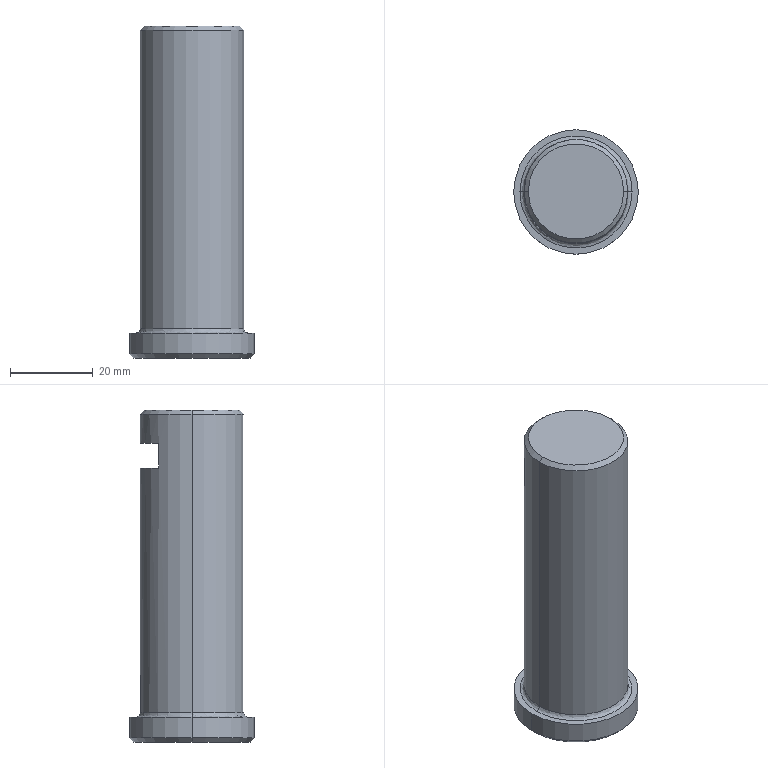Part | STEP file | 1 solid | 16 faces | box 30 x 30 x 80 mm | volume 40134 mm3 | plane 6 | cone 4 | cylinder 4 | spline 2 | commonest cylinder face diameters 25 x2 30 x2